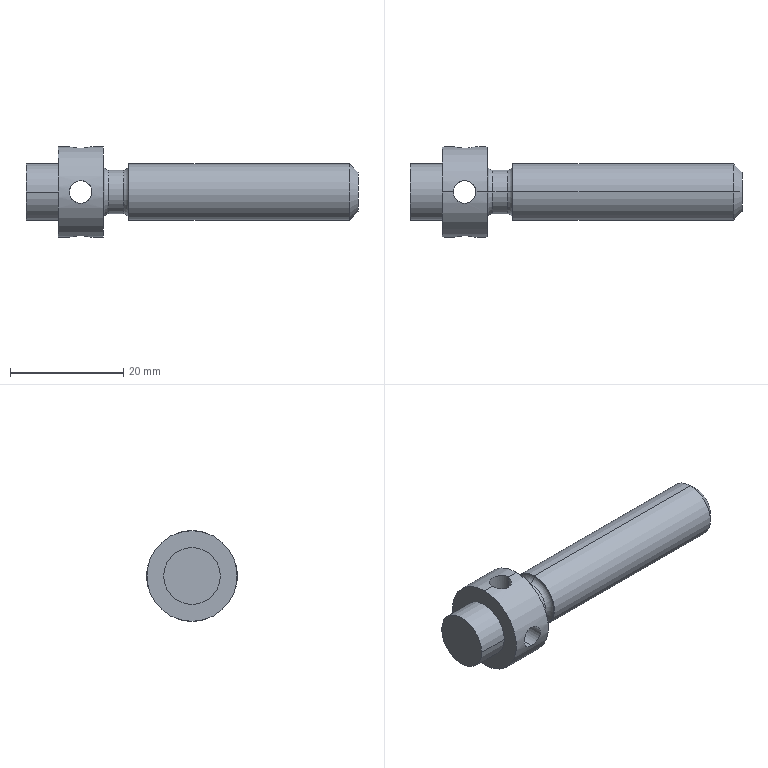Part | SolidWorks | features Boss 2, Cut 2, Chamfer 1, Extrusion 1, Fillet 1, ICE 1, Revolution 1 | 1 solid | 27 faces | box 58.66 x 16 x 16 mm | volume 5066 mm3 | cylinder 16 | plane 5 | torus 4 | cone 2 | commonest cylinder face diameters 4 x8 10 x4 7.7 x2 16 x2
STEP:
#1=CARTESIAN_POINT('',(-40.5,0.,4.85));
#2=VERTEX_POINT('',#1);
#3=CARTESIAN_POINT('',(-40.5,0.,-4.85));
#4=VERTEX_POINT('',#3);
#5=CARTESIAN_POINT('',(-40.5,0.,0.));
#6=DIRECTION('',(1.,0.,0.));
#7=DIRECTION('',(0.,0.,-1.));
#8=AXIS2_PLACEMENT_3D('',#5,#6,#7);
#9=CIRCLE('',#8,4.85);
#10=EDGE_CURVE('',#2,#4,#9,.T.);
#11=ORIENTED_EDGE('',*,*,#10,.F.);
#12=CARTESIAN_POINT('',(-41.5,0.,3.85));
#13=VERTEX_POINT('',#12);
#14=CARTESIAN_POINT('',(-41.5,0.,4.85));
#15=DIRECTION('',(0.,1.,0.));
#16=DIRECTION('',(0.,0.,1.));
#17=AXIS2_PLACEMENT_3D('',#14,#15,#16);
#18=CIRCLE('',#17,1.);
#19=EDGE_CURVE('',#2,#13,#18,.T.);
#20=ORIENTED_EDGE('',*,*,#19,.T.);
#21=CARTESIAN_POINT('',(-41.5,0.,-3.85));
#22=VERTEX_POINT('',#21);
#23=CARTESIAN_POINT('',(-41.5,0.,0.));
#24=DIRECTION('',(-1.,0.,0.));
#25=DIRECTION('',(0.,0.,-1.));
#26=AXIS2_PLACEMENT_3D('',#23,#24,#25);
#27=CIRCLE('',#26,3.85);
#28=EDGE_CURVE('',#22,#13,#27,.T.);
#29=ORIENTED_EDGE('',*,*,#28,.F.);
#30=CARTESIAN_POINT('',(-41.5,0.,-4.85));
#31=DIRECTION('',(0.,-1.,0.));
#32=DIRECTION('',(1.,0.,0.));
#33=AXIS2_PLACEMENT_3D('',#30,#31,#32);
#34=CIRCLE('',#33,1.);
#35=EDGE_CURVE('',#4,#22,#34,.T.);
#36=ORIENTED_EDGE('',*,*,#35,.F.);
#37=EDGE_LOOP('',(#11,#20,#29,#36));
#38=FACE_OUTER_BOUND('',#37,.T.);
#39=CARTESIAN_POINT('',(-41.5,0.,0.));
#40=DIRECTION('',(1.,0.,0.));
#41=DIRECTION('',(0.,0.,-1.));
#42=AXIS2_PLACEMENT_3D('',#39,#40,#41);
#43=TOROIDAL_SURFACE('',#42,4.85,1.);
#44=ADVANCED_FACE('',(#38),#43,.F.);
#45=CARTESIAN_POINT('',(-45.,0.,-4.85));
#46=VERTEX_POINT('',#45);
#47=CARTESIAN_POINT('',(-45.,0.,4.85));
#48=VERTEX_POINT('',#47);
#49=CARTESIAN_POINT('',(-45.,0.,0.));
#50=DIRECTION('',(-1.,0.,0.));
#51=DIRECTION('',(0.,0.,1.));
#52=AXIS2_PLACEMENT_3D('',#49,#50,#51);
#53=CIRCLE('',#52,4.85);
#54=EDGE_CURVE('',#46,#48,#53,.T.);
#55=ORIENTED_EDGE('',*,*,#54,.F.);
#56=CARTESIAN_POINT('',(-44.,0.,-3.85));
#57=VERTEX_POINT('',#56);
#58=CARTESIAN_POINT('',(-44.,0.,-4.85));
#59=DIRECTION('',(0.,1.,0.));
#60=DIRECTION('',(0.,0.,1.));
#61=AXIS2_PLACEMENT_3D('',#58,#59,#60);
#62=CIRCLE('',#61,1.);
#63=EDGE_CURVE('',#46,#57,#62,.T.);
#64=ORIENTED_EDGE('',*,*,#63,.T.);
#65=CARTESIAN_POINT('',(-44.,0.,3.85));
#66=VERTEX_POINT('',#65);
#67=CARTESIAN_POINT('',(-44.,0.,0.));
#68=DIRECTION('',(1.,0.,0.));
#69=DIRECTION('',(0.,0.,1.));
#70=AXIS2_PLACEMENT_3D('',#67,#68,#69);
#71=CIRCLE('',#70,3.85);
#72=EDGE_CURVE('',#66,#57,#71,.T.);
#73=ORIENTED_EDGE('',*,*,#72,.F.);
#74=CARTESIAN_POINT('',(-44.,0.,4.85));
#75=DIRECTION('',(0.,-1.,0.));
#76=DIRECTION('',(1.,0.,0.));
#77=AXIS2_PLACEMENT_3D('',#74,#75,#76);
#78=CIRCLE('',#77,1.);
#79=EDGE_CURVE('',#48,#66,#78,.T.);
#80=ORIENTED_EDGE('',*,*,#79,.F.);
#81=EDGE_LOOP('',(#55,#64,#73,#80));
#82=FACE_OUTER_BOUND('',#81,.T.);
#83=CARTESIAN_POINT('',(-44.,0.,0.));
#84=DIRECTION('',(-1.,0.,0.));
#85=DIRECTION('',(0.,0.,1.));
#86=AXIS2_PLACEMENT_3D('',#83,#84,#85);
#87=TOROIDAL_SURFACE('',#86,4.85,1.);
#88=ADVANCED_FACE('',(#82),#87,.F.);
#89=CARTESIAN_POINT('',(-58.66,-5.,0.));
#90=VERTEX_POINT('',#89);
#91=CARTESIAN_POINT('',(-58.66,5.,0.));
#92=VERTEX_POINT('',#91);
#93=CARTESIAN_POINT('',(-58.66,0.,0.));
#94=DIRECTION('',(-1.,0.,0.));
#95=DIRECTION('',(0.,0.,-1.));
#96=AXIS2_PLACEMENT_3D('',#93,#94,#95);
#97=CIRCLE('',#96,5.);
#98=EDGE_CURVE('',#90,#92,#97,.T.);
#99=ORIENTED_EDGE('',*,*,#98,.F.);
#100=CARTESIAN_POINT('',(-53.,-5.,0.));
#101=VERTEX_POINT('',#100);
#102=CARTESIAN_POINT('',(-53.,-5.,0.));
#103=DIRECTION('',(1.,0.,0.));
#104=VECTOR('',#103,1000.);
#105=LINE('',#102,#104);
#106=EDGE_CURVE('',#90,#101,#105,.T.);
#107=ORIENTED_EDGE('',*,*,#106,.T.);
#108=CARTESIAN_POINT('',(-53.,5.,0.));
#109=VERTEX_POINT('',#108);
#110=CARTESIAN_POINT('',(-53.,0.,0.));
#111=DIRECTION('',(-1.,0.,0.));
#112=DIRECTION('',(0.,0.,1.));
#113=AXIS2_PLACEMENT_3D('',#110,#111,#112);
#114=CIRCLE('',#113,5.);
#115=EDGE_CURVE('',#101,#109,#114,.T.);
#116=ORIENTED_EDGE('',*,*,#115,.T.);
#117=CARTESIAN_POINT('',(-53.,5.,0.));
#118=DIRECTION('',(1.,0.,0.));
#119=VECTOR('',#118,1000.);
#120=LINE('',#117,#119);
#121=EDGE_CURVE('',#92,#109,#120,.T.);
#122=ORIENTED_EDGE('',*,*,#121,.F.);
#123=EDGE_LOOP('',(#99,#107,#116,#122));
#124=FACE_OUTER_BOUND('',#123,.T.);
#125=CARTESIAN_POINT('',(-53.,0.,0.));
#126=DIRECTION('',(1.,0.,0.));
#127=DIRECTION('',(0.,1.,0.));
#128=AXIS2_PLACEMENT_3D('',#125,#126,#127);
#129=CYLINDRICAL_SURFACE('',#128,5.);
#130=ADVANCED_FACE('',(#124),#129,.T.);
#131=CARTESIAN_POINT('',(-49.,-7.746,-2.));
#132=VERTEX_POINT('',#131);
#133=CARTESIAN_POINT('',(-49.,-7.746,2.));
#134=VERTEX_POINT('',#133);
#135=CARTESIAN_POINT('',(-49.,-7.746,-2.));
#136=CARTESIAN_POINT('',(-49.131,-7.746,-2.));
#137=CARTESIAN_POINT('',(-49.264,-7.749,-1.987));
#138=CARTESIAN_POINT('',(-49.521,-7.762,-1.935));
#139=CARTESIAN_POINT('',(-49.646,-7.772,-1.897));
#140=CARTESIAN_POINT('',(-50.01,-7.808,-1.746));
#141=CARTESIAN_POINT('',(-50.23,-7.841,-1.599));
#142=CARTESIAN_POINT('',(-50.508,-7.891,-1.321));
#143=CARTESIAN_POINT('',(-50.59,-7.907,-1.22));
#144=CARTESIAN_POINT('',(-50.735,-7.937,-1.004));
#145=CARTESIAN_POINT('',(-50.797,-7.952,-0.887));
#146=CARTESIAN_POINT('',(-50.897,-7.975,-0.6456));
#147=CARTESIAN_POINT('',(-50.935,-7.984,-0.5209));
#148=CARTESIAN_POINT('',(-50.987,-7.997,-0.2633));
#149=CARTESIAN_POINT('',(-51.,-8.,-0.1305));
#150=CARTESIAN_POINT('',(-51.,-8.,0.2619));
#151=CARTESIAN_POINT('',(-50.947,-7.986,0.5261));
#152=CARTESIAN_POINT('',(-50.797,-7.952,0.8874));
#153=CARTESIAN_POINT('',(-50.734,-7.937,1.004));
#154=CARTESIAN_POINT('',(-50.589,-7.907,1.221));
#155=CARTESIAN_POINT('',(-50.507,-7.891,1.322));
#156=CARTESIAN_POINT('',(-50.322,-7.857,1.506));
#157=CARTESIAN_POINT('',(-50.22,-7.841,1.59));
#158=CARTESIAN_POINT('',(-50.004,-7.81,1.735));
#159=CARTESIAN_POINT('',(-49.889,-7.796,1.796));
#160=CARTESIAN_POINT('',(-49.524,-7.76,1.948));
#161=CARTESIAN_POINT('',(-49.264,-7.746,2.));
#162=CARTESIAN_POINT('',(-49.,-7.746,2.));
#163=B_SPLINE_CURVE_WITH_KNOTS('',3,(#135,#136,#137,#138,#139,#140,#141,#142,#143,#144,#145,#146,#147,#148,#149,#150,#151,#152,#153,#154,#155,#156,#157,#158,#159,#160,#161,#162),.UNSPECIFIED.,.F.,.F.,(4,2,2,2,2,2,2,2,2,2,2,2,2,4),(0.00314,0.003532,0.003924,0.004709,0.005101,0.005494,0.005886,0.006278,0.007063,0.007455,0.007847,0.00824,0.008632,0.009417),.UNSPECIFIED.);
#164=EDGE_CURVE('',#132,#134,#163,.T.);
#165=ORIENTED_EDGE('',*,*,#164,.F.);
#166=CARTESIAN_POINT('',(-49.,-2.,-2.));
#167=VERTEX_POINT('',#166);
#168=CARTESIAN_POINT('',(-49.,-8.,-2.));
#169=DIRECTION('',(0.,1.,0.));
#170=VECTOR('',#169,1000.);
#171=LINE('',#168,#170);
#172=EDGE_CURVE('',#132,#167,#171,.T.);
#173=ORIENTED_EDGE('',*,*,#172,.T.);
#174=CARTESIAN_POINT('',(-51.,0.,0.));
#175=VERTEX_POINT('',#174);
#176=CARTESIAN_POINT('',(-51.,0.,0.));
#177=CARTESIAN_POINT('',(-51.,-1.172,-1.172));
#178=CARTESIAN_POINT('',(-50.172,-2.,-2.));
#179=CARTESIAN_POINT('',(-49.,-2.,-2.));
#180=(BOUNDED_CURVE()B_SPLINE_CURVE(3,(#176,#177,#178,#179),.UNSPECIFIED.,.F.,.T.)B_SPLINE_CURVE_WITH_KNOTS((4,4),(1.571,3.142),.UNSPECIFIED.)CURVE()GEOMETRIC_REPRESENTATION_ITEM()RATIONAL_B_SPLINE_CURVE((1.,0.8047,0.8047,1.))REPRESENTATION_ITEM(''));
#181=EDGE_CURVE('',#175,#167,#180,.T.);
#182=ORIENTED_EDGE('',*,*,#181,.F.);
#183=CARTESIAN_POINT('',(-49.,-2.,2.));
#184=VERTEX_POINT('',#183);
#185=CARTESIAN_POINT('',(-49.,-2.,2.));
#186=CARTESIAN_POINT('',(-50.172,-2.,2.));
#187=CARTESIAN_POINT('',(-51.,-1.172,1.172));
#188=CARTESIAN_POINT('',(-51.,0.,0.));
#189=(BOUNDED_CURVE()B_SPLINE_CURVE(3,(#185,#186,#187,#188),.UNSPECIFIED.,.F.,.F.)B_SPLINE_CURVE_WITH_KNOTS((4,4),(0.,1.571),.UNSPECIFIED.)CURVE()GEOMETRIC_REPRESENTATION_ITEM()RATIONAL_B_SPLINE_CURVE((1.,0.8047,0.8047,1.))REPRESENTATION_ITEM(''));
#190=EDGE_CURVE('',#184,#175,#189,.T.);
#191=ORIENTED_EDGE('',*,*,#190,.F.);
#192=CARTESIAN_POINT('',(-49.,-8.,2.));
#193=DIRECTION('',(0.,1.,0.));
#194=VECTOR('',#193,1000.);
#195=LINE('',#192,#194);
#196=EDGE_CURVE('',#134,#184,#195,.T.);
#197=ORIENTED_EDGE('',*,*,#196,.F.);
#198=EDGE_LOOP('',(#165,#173,#182,#191,#197));
#199=FACE_OUTER_BOUND('',#198,.T.);
#200=CARTESIAN_POINT('',(-49.,-8.,0.));
#201=DIRECTION('',(0.,1.,0.));
#202=DIRECTION('',(0.,0.,1.));
#203=AXIS2_PLACEMENT_3D('',#200,#201,#202);
#204=CYLINDRICAL_SURFACE('',#203,2.);
#205=ADVANCED_FACE('',(#199),#204,.F.);
#206=CARTESIAN_POINT('',(-49.,2.,-2.));
#207=VERTEX_POINT('',#206);
#208=CARTESIAN_POINT('',(-49.,2.,-2.));
#209=CARTESIAN_POINT('',(-50.172,2.,-2.));
#210=CARTESIAN_POINT('',(-51.,1.172,-1.172));
#211=CARTESIAN_POINT('',(-51.,0.,0.));
#212=(BOUNDED_CURVE()B_SPLINE_CURVE(3,(#208,#209,#210,#211),.UNSPECIFIED.,.F.,.F.)B_SPLINE_CURVE_WITH_KNOTS((4,4),(3.142,4.712),.UNSPECIFIED.)CURVE()GEOMETRIC_REPRESENTATION_ITEM()RATIONAL_B_SPLINE_CURVE((1.,0.8047,0.8047,1.))REPRESENTATION_ITEM(''));
#213=EDGE_CURVE('',#207,#175,#212,.T.);
#214=ORIENTED_EDGE('',*,*,#213,.F.);
#215=CARTESIAN_POINT('',(-49.,7.746,-2.));
#216=VERTEX_POINT('',#215);
#217=CARTESIAN_POINT('',(-49.,-8.,-2.));
#218=DIRECTION('',(0.,1.,0.));
#219=VECTOR('',#218,1000.);
#220=LINE('',#217,#219);
#221=EDGE_CURVE('',#207,#216,#220,.T.);
#222=ORIENTED_EDGE('',*,*,#221,.T.);
#223=CARTESIAN_POINT('',(-49.,7.746,2.));
#224=VERTEX_POINT('',#223);
#225=CARTESIAN_POINT('',(-49.,7.746,2.));
#226=CARTESIAN_POINT('',(-49.133,7.746,2.));
#227=CARTESIAN_POINT('',(-49.263,7.749,1.987));
#228=CARTESIAN_POINT('',(-49.519,7.762,1.936));
#229=CARTESIAN_POINT('',(-49.647,7.772,1.897));
#230=CARTESIAN_POINT('',(-49.889,7.796,1.796));
#231=CARTESIAN_POINT('',(-50.003,7.81,1.735));
#232=CARTESIAN_POINT('',(-50.22,7.841,1.59));
#233=CARTESIAN_POINT('',(-50.323,7.858,1.506));
#234=CARTESIAN_POINT('',(-50.598,7.907,1.23));
#235=CARTESIAN_POINT('',(-50.747,7.94,1.008));
#236=CARTESIAN_POINT('',(-50.897,7.975,0.6471));
#237=CARTESIAN_POINT('',(-50.936,7.984,0.5204));
#238=CARTESIAN_POINT('',(-50.987,7.997,0.262));
#239=CARTESIAN_POINT('',(-51.,8.,0.1319));
#240=CARTESIAN_POINT('',(-51.,8.,-0.1302));
#241=CARTESIAN_POINT('',(-50.987,7.997,-0.2634));
#242=CARTESIAN_POINT('',(-50.936,7.984,-0.5203));
#243=CARTESIAN_POINT('',(-50.898,7.975,-0.6453));
#244=CARTESIAN_POINT('',(-50.746,7.94,-1.01));
#245=CARTESIAN_POINT('',(-50.599,7.907,-1.229));
#246=CARTESIAN_POINT('',(-50.321,7.857,-1.507));
#247=CARTESIAN_POINT('',(-50.221,7.841,-1.59));
#248=CARTESIAN_POINT('',(-50.004,7.81,-1.734));
#249=CARTESIAN_POINT('',(-49.887,7.796,-1.797));
#250=CARTESIAN_POINT('',(-49.646,7.772,-1.897));
#251=CARTESIAN_POINT('',(-49.521,7.762,-1.935));
#252=CARTESIAN_POINT('',(-49.264,7.749,-1.987));
#253=CARTESIAN_POINT('',(-49.131,7.746,-2.));
#254=CARTESIAN_POINT('',(-49.,7.746,-2.));
#255=B_SPLINE_CURVE_WITH_KNOTS('',3,(#225,#226,#227,#228,#229,#230,#231,#232,#233,#234,#235,#236,#237,#238,#239,#240,#241,#242,#243,#244,#245,#246,#247,#248,#249,#250,#251,#252,#253,#254),.UNSPECIFIED.,.F.,.F.,(4,2,2,2,2,2,2,2,2,2,2,2,2,2,4),(0.,0.0003924,0.0007847,0.001177,0.001569,0.002354,0.002747,0.003139,0.003531,0.003924,0.004708,0.005101,0.005493,0.005885,0.006278),.UNSPECIFIED.);
#256=EDGE_CURVE('',#224,#216,#255,.T.);
#257=ORIENTED_EDGE('',*,*,#256,.F.);
#258=CARTESIAN_POINT('',(-49.,2.,2.));
#259=VERTEX_POINT('',#258);
#260=CARTESIAN_POINT('',(-49.,-8.,2.));
#261=DIRECTION('',(0.,1.,0.));
#262=VECTOR('',#261,1000.);
#263=LINE('',#260,#262);
#264=EDGE_CURVE('',#259,#224,#263,.T.);
#265=ORIENTED_EDGE('',*,*,#264,.F.);
#266=CARTESIAN_POINT('',(-51.,0.,0.));
#267=CARTESIAN_POINT('',(-51.,1.172,1.172));
#268=CARTESIAN_POINT('',(-50.172,2.,2.));
#269=CARTESIAN_POINT('',(-49.,2.,2.));
#270=(BOUNDED_CURVE()B_SPLINE_CURVE(3,(#266,#267,#268,#269),.UNSPECIFIED.,.F.,.F.)B_SPLINE_CURVE_WITH_KNOTS((4,4),(4.712,6.283),.UNSPECIFIED.)CURVE()GEOMETRIC_REPRESENTATION_ITEM()RATIONAL_B_SPLINE_CURVE((1.,0.8047,0.8047,1.))REPRESENTATION_ITEM(''));
#271=EDGE_CURVE('',#175,#259,#270,.T.);
#272=ORIENTED_EDGE('',*,*,#271,.F.);
#273=EDGE_LOOP('',(#214,#222,#257,#265,#272));
#274=FACE_OUTER_BOUND('',#273,.T.);
#275=CARTESIAN_POINT('',(-49.,-8.,0.));
#276=DIRECTION('',(0.,1.,0.));
#277=DIRECTION('',(0.,0.,1.));
#278=AXIS2_PLACEMENT_3D('',#275,#276,#277);
#279=CYLINDRICAL_SURFACE('',#278,2.);
#280=ADVANCED_FACE('',(#274),#279,.F.);
#281=CARTESIAN_POINT('',(-51.,0.,-8.));
#282=VERTEX_POINT('',#281);
#283=CARTESIAN_POINT('',(-47.,0.,-8.));
#284=VERTEX_POINT('',#283);
#285=CARTESIAN_POINT('',(-51.,0.,-8.));
#286=CARTESIAN_POINT('',(-51.,-0.2616,-8.));
#287=CARTESIAN_POINT('',(-50.947,-0.5257,-7.986));
#288=CARTESIAN_POINT('',(-50.797,-0.8871,-7.952));
#289=CARTESIAN_POINT('',(-50.735,-1.004,-7.937));
#290=CARTESIAN_POINT('',(-50.589,-1.221,-7.907));
#291=CARTESIAN_POINT('',(-50.507,-1.321,-7.891));
#292=CARTESIAN_POINT('',(-50.323,-1.506,-7.858));
#293=CARTESIAN_POINT('',(-50.22,-1.59,-7.841));
#294=CARTESIAN_POINT('',(-50.004,-1.734,-7.81));
#295=CARTESIAN_POINT('',(-49.89,-1.796,-7.796));
#296=CARTESIAN_POINT('',(-49.525,-1.948,-7.76));
#297=CARTESIAN_POINT('',(-49.264,-2.,-7.746));
#298=CARTESIAN_POINT('',(-48.869,-2.,-7.746));
#299=CARTESIAN_POINT('',(-48.739,-1.987,-7.749));
#300=CARTESIAN_POINT('',(-48.482,-1.936,-7.762));
#301=CARTESIAN_POINT('',(-48.354,-1.897,-7.772));
#302=CARTESIAN_POINT('',(-47.992,-1.747,-7.808));
#303=CARTESIAN_POINT('',(-47.77,-1.598,-7.841));
#304=CARTESIAN_POINT('',(-47.403,-1.232,-7.907));
#305=CARTESIAN_POINT('',(-47.254,-1.01,-7.94));
#306=CARTESIAN_POINT('',(-47.104,-0.6486,-7.975));
#307=CARTESIAN_POINT('',(-47.065,-0.5212,-7.984));
#308=CARTESIAN_POINT('',(-47.013,-0.2634,-7.997));
#309=CARTESIAN_POINT('',(-47.,-0.1327,-8.));
#310=CARTESIAN_POINT('',(-47.,0.,-8.));
#311=B_SPLINE_CURVE_WITH_KNOTS('',3,(#285,#286,#287,#288,#289,#290,#291,#292,#293,#294,#295,#296,#297,#298,#299,#300,#301,#302,#303,#304,#305,#306,#307,#308,#309,#310),.UNSPECIFIED.,.F.,.F.,(4,2,2,2,2,2,2,2,2,2,2,2,4),(0.006278,0.007062,0.007455,0.007847,0.008239,0.008631,0.009416,0.009808,0.0102,0.01099,0.01177,0.01216,0.01255),.UNSPECIFIED.);
#312=EDGE_CURVE('',#282,#284,#311,.T.);
#313=ORIENTED_EDGE('',*,*,#312,.F.);
#314=CARTESIAN_POINT('',(-51.,0.,-8.));
#315=DIRECTION('',(0.,0.,1.));
#316=VECTOR('',#315,1000.);
#317=LINE('',#314,#316);
#318=EDGE_CURVE('',#282,#175,#317,.T.);
#319=ORIENTED_EDGE('',*,*,#318,.T.);
#320=ORIENTED_EDGE('',*,*,#181,.T.);
#321=CARTESIAN_POINT('',(-47.,0.,0.));
#322=VERTEX_POINT('',#321);
#323=CARTESIAN_POINT('',(-49.,-2.,-2.));
#324=CARTESIAN_POINT('',(-47.828,-2.,-2.));
#325=CARTESIAN_POINT('',(-47.,-1.172,-1.172));
#326=CARTESIAN_POINT('',(-47.,0.,0.));
#327=(BOUNDED_CURVE()B_SPLINE_CURVE(3,(#323,#324,#325,#326),.UNSPECIFIED.,.F.,.T.)B_SPLINE_CURVE_WITH_KNOTS((4,4),(3.142,4.712),.UNSPECIFIED.)CURVE()GEOMETRIC_REPRESENTATION_ITEM()RATIONAL_B_SPLINE_CURVE((1.,0.8047,0.8047,1.))REPRESENTATION_ITEM(''));
#328=EDGE_CURVE('',#167,#322,#327,.T.);
#329=ORIENTED_EDGE('',*,*,#328,.T.);
#330=CARTESIAN_POINT('',(-47.,0.,-8.));
#331=DIRECTION('',(0.,0.,1.));
#332=VECTOR('',#331,1000.);
#333=LINE('',#330,#332);
#334=EDGE_CURVE('',#284,#322,#333,.T.);
#335=ORIENTED_EDGE('',*,*,#334,.F.);
#336=EDGE_LOOP('',(#313,#319,#320,#329,#335));
#337=FACE_OUTER_BOUND('',#336,.T.);
#338=CARTESIAN_POINT('',(-49.,0.,-8.));
#339=DIRECTION('',(0.,0.,1.));
#340=DIRECTION('',(1.,0.,0.));
#341=AXIS2_PLACEMENT_3D('',#338,#339,#340);
#342=CYLINDRICAL_SURFACE('',#341,2.);
#343=ADVANCED_FACE('',(#337),#342,.F.);
#344=ORIENTED_EDGE('',*,*,#256,.T.);
#345=CARTESIAN_POINT('',(-49.,7.746,-2.));
#346=CARTESIAN_POINT('',(-48.738,7.746,-2.));
#347=CARTESIAN_POINT('',(-48.474,7.76,-1.947));
#348=CARTESIAN_POINT('',(-48.113,7.796,-1.797));
#349=CARTESIAN_POINT('',(-47.996,7.81,-1.735));
#350=CARTESIAN_POINT('',(-47.779,7.841,-1.589));
#351=CARTESIAN_POINT('',(-47.679,7.857,-1.507));
#352=CARTESIAN_POINT('',(-47.494,7.89,-1.323));
#353=CARTESIAN_POINT('',(-47.41,7.907,-1.22));
#354=CARTESIAN_POINT('',(-47.266,7.937,-1.004));
#355=CARTESIAN_POINT('',(-47.204,7.951,-0.8897));
#356=CARTESIAN_POINT('',(-47.052,7.987,-0.5248));
#357=CARTESIAN_POINT('',(-47.,8.,-0.2644));
#358=CARTESIAN_POINT('',(-47.,8.,0.1313));
#359=CARTESIAN_POINT('',(-47.013,7.997,0.2615));
#360=CARTESIAN_POINT('',(-47.064,7.984,0.5184));
#361=CARTESIAN_POINT('',(-47.103,7.975,0.646));
#362=CARTESIAN_POINT('',(-47.253,7.94,1.008));
#363=CARTESIAN_POINT('',(-47.402,7.907,1.23));
#364=CARTESIAN_POINT('',(-47.769,7.841,1.597));
#365=CARTESIAN_POINT('',(-47.99,7.808,1.746));
#366=CARTESIAN_POINT('',(-48.351,7.772,1.896));
#367=CARTESIAN_POINT('',(-48.479,7.762,1.935));
#368=CARTESIAN_POINT('',(-48.737,7.749,1.987));
#369=CARTESIAN_POINT('',(-48.867,7.746,2.));
#370=CARTESIAN_POINT('',(-49.,7.746,2.));
#371=B_SPLINE_CURVE_WITH_KNOTS('',3,(#345,#346,#347,#348,#349,#350,#351,#352,#353,#354,#355,#356,#357,#358,#359,#360,#361,#362,#363,#364,#365,#366,#367,#368,#369,#370),.UNSPECIFIED.,.F.,.F.,(4,2,2,2,2,2,2,2,2,2,2,2,4),(0.006278,0.007062,0.007455,0.007847,0.008239,0.008631,0.009416,0.009808,0.0102,0.01098,0.01177,0.01216,0.01255),.UNSPECIFIED.);
#372=EDGE_CURVE('',#216,#224,#371,.T.);
#373=ORIENTED_EDGE('',*,*,#372,.T.);
#374=EDGE_LOOP('',(#344,#373));
#375=FACE_BOUND('',#374,.T.);
#376=CARTESIAN_POINT('',(-53.,0.,8.));
#377=VERTEX_POINT('',#376);
#378=CARTESIAN_POINT('',(-53.,0.,-8.));
#379=VERTEX_POINT('',#378);
#380=CARTESIAN_POINT('',(-53.,0.,0.));
#381=DIRECTION('',(-1.,0.,0.));
#382=DIRECTION('',(0.,0.,1.));
#383=AXIS2_PLACEMENT_3D('',#380,#381,#382);
#384=CIRCLE('',#383,8.);
#385=EDGE_CURVE('',#377,#379,#384,.T.);
#386=ORIENTED_EDGE('',*,*,#385,.F.);
#387=CARTESIAN_POINT('',(-51.,0.,8.));
#388=VERTEX_POINT('',#387);
#389=CARTESIAN_POINT('',(-53.,0.,8.));
#390=DIRECTION('',(1.,0.,0.));
#391=VECTOR('',#390,1000.);
#392=LINE('',#389,#391);
#393=EDGE_CURVE('',#377,#388,#392,.T.);
#394=ORIENTED_EDGE('',*,*,#393,.T.);
#395=CARTESIAN_POINT('',(-47.,0.,8.));
#396=VERTEX_POINT('',#395);
#397=CARTESIAN_POINT('',(-51.,0.,8.));
#398=CARTESIAN_POINT('',(-51.,0.2616,8.));
#399=CARTESIAN_POINT('',(-50.947,0.5257,7.986));
#400=CARTESIAN_POINT('',(-50.797,0.8871,7.952));
#401=CARTESIAN_POINT('',(-50.735,1.004,7.937));
#402=CARTESIAN_POINT('',(-50.589,1.221,7.907));
#403=CARTESIAN_POINT('',(-50.507,1.321,7.891));
#404=CARTESIAN_POINT('',(-50.323,1.506,7.858));
#405=CARTESIAN_POINT('',(-50.22,1.59,7.841));
#406=CARTESIAN_POINT('',(-50.004,1.734,7.81));
#407=CARTESIAN_POINT('',(-49.89,1.796,7.796));
#408=CARTESIAN_POINT('',(-49.525,1.948,7.76));
#409=CARTESIAN_POINT('',(-49.264,2.,7.746));
#410=CARTESIAN_POINT('',(-48.869,2.,7.746));
#411=CARTESIAN_POINT('',(-48.739,1.987,7.749));
#412=CARTESIAN_POINT('',(-48.482,1.936,7.762));
#413=CARTESIAN_POINT('',(-48.354,1.897,7.772));
#414=CARTESIAN_POINT('',(-47.992,1.747,7.808));
#415=CARTESIAN_POINT('',(-47.77,1.598,7.841));
#416=CARTESIAN_POINT('',(-47.403,1.232,7.907));
#417=CARTESIAN_POINT('',(-47.254,1.01,7.94));
#418=CARTESIAN_POINT('',(-47.104,0.6486,7.975));
#419=CARTESIAN_POINT('',(-47.065,0.5212,7.984));
#420=CARTESIAN_POINT('',(-47.013,0.2634,7.997));
#421=CARTESIAN_POINT('',(-47.,0.1327,8.));
#422=CARTESIAN_POINT('',(-47.,0.,8.));
#423=B_SPLINE_CURVE_WITH_KNOTS('',3,(#397,#398,#399,#400,#401,#402,#403,#404,#405,#406,#407,#408,#409,#410,#411,#412,#413,#414,#415,#416,#417,#418,#419,#420,#421,#422),.UNSPECIFIED.,.F.,.F.,(4,2,2,2,2,2,2,2,2,2,2,2,4),(0.006278,0.007062,0.007455,0.007847,0.008239,0.008631,0.009416,0.009808,0.0102,0.01099,0.01177,0.01216,0.01255),.UNSPECIFIED.);
#424=EDGE_CURVE('',#388,#396,#423,.T.);
#425=ORIENTED_EDGE('',*,*,#424,.T.);
#426=CARTESIAN_POINT('',(-45.,0.,8.));
#427=VERTEX_POINT('',#426);
#428=CARTESIAN_POINT('',(-53.,0.,8.));
#429=DIRECTION('',(1.,0.,0.));
#430=VECTOR('',#429,1000.);
#431=LINE('',#428,#430);
#432=EDGE_CURVE('',#396,#427,#431,.T.);
#433=ORIENTED_EDGE('',*,*,#432,.T.);
#434=CARTESIAN_POINT('',(-45.,0.,-8.));
#435=VERTEX_POINT('',#434);
#436=CARTESIAN_POINT('',(-45.,0.,0.));
#437=DIRECTION('',(-1.,0.,0.));
#438=DIRECTION('',(0.,0.,1.));
#439=AXIS2_PLACEMENT_3D('',#436,#437,#438);
#440=CIRCLE('',#439,8.);
#441=EDGE_CURVE('',#427,#435,#440,.T.);
#442=ORIENTED_EDGE('',*,*,#441,.T.);
#443=CARTESIAN_POINT('',(-53.,0.,-8.));
#444=DIRECTION('',(1.,0.,0.));
#445=VECTOR('',#444,1000.);
#446=LINE('',#443,#445);
#447=EDGE_CURVE('',#284,#435,#446,.T.);
#448=ORIENTED_EDGE('',*,*,#447,.F.);
#449=CARTESIAN_POINT('',(-47.,0.,-8.));
#450=CARTESIAN_POINT('',(-47.,0.1327,-8.));
#451=CARTESIAN_POINT('',(-47.013,0.2631,-7.997));
#452=CARTESIAN_POINT('',(-47.064,0.5195,-7.984));
#453=CARTESIAN_POINT('',(-47.103,0.6468,-7.975));
#454=CARTESIAN_POINT('',(-47.204,0.8888,-7.951));
#455=CARTESIAN_POINT('',(-47.265,1.003,-7.938));
#456=CARTESIAN_POINT('',(-47.41,1.22,-7.907));
#457=CARTESIAN_POINT('',(-47.494,1.323,-7.89));
#458=CARTESIAN_POINT('',(-47.77,1.598,-7.841));
#459=CARTESIAN_POINT('',(-47.992,1.747,-7.808));
#460=CARTESIAN_POINT('',(-48.353,1.897,-7.772));
#461=CARTESIAN_POINT('',(-48.48,1.936,-7.762));
#462=CARTESIAN_POINT('',(-48.738,1.987,-7.749));
#463=CARTESIAN_POINT('',(-48.868,2.,-7.746));
#464=CARTESIAN_POINT('',(-49.13,2.,-7.746));
#465=CARTESIAN_POINT('',(-49.263,1.987,-7.749));
#466=CARTESIAN_POINT('',(-49.52,1.936,-7.762));
#467=CARTESIAN_POINT('',(-49.645,1.898,-7.772));
#468=CARTESIAN_POINT('',(-50.009,1.746,-7.808));
#469=CARTESIAN_POINT('',(-50.229,1.599,-7.841));
#470=CARTESIAN_POINT('',(-50.507,1.321,-7.891));
#471=CARTESIAN_POINT('',(-50.59,1.221,-7.907));
#472=CARTESIAN_POINT('',(-50.734,1.005,-7.937));
#473=CARTESIAN_POINT('',(-50.797,0.8874,-7.952));
#474=CARTESIAN_POINT('',(-50.897,0.646,-7.975));
#475=CARTESIAN_POINT('',(-50.935,0.5212,-7.984));
#476=CARTESIAN_POINT('',(-50.987,0.2636,-7.997));
#477=CARTESIAN_POINT('',(-51.,0.1308,-8.));
#478=CARTESIAN_POINT('',(-51.,0.,-8.));
#479=B_SPLINE_CURVE_WITH_KNOTS('',3,(#449,#450,#451,#452,#453,#454,#455,#456,#457,#458,#459,#460,#461,#462,#463,#464,#465,#466,#467,#468,#469,#470,#471,#472,#473,#474,#475,#476,#477,#478),.UNSPECIFIED.,.F.,.F.,(4,2,2,2,2,2,2,2,2,2,2,2,2,2,4),(0.,0.0003924,0.0007847,0.001177,0.001569,0.002354,0.002747,0.003139,0.003531,0.003924,0.004708,0.005101,0.005493,0.005886,0.006278),.UNSPECIFIED.);
#480=EDGE_CURVE('',#284,#282,#479,.T.);
#481=ORIENTED_EDGE('',*,*,#480,.T.);
#482=CARTESIAN_POINT('',(-53.,0.,-8.));
#483=DIRECTION('',(1.,0.,0.));
#484=VECTOR('',#483,1000.);
#485=LINE('',#482,#484);
#486=EDGE_CURVE('',#379,#282,#485,.T.);
#487=ORIENTED_EDGE('',*,*,#486,.F.);
#488=EDGE_LOOP('',(#386,#394,#425,#433,#442,#448,#481,#487));
#489=FACE_OUTER_BOUND('',#488,.T.);
#490=CARTESIAN_POINT('',(-53.,0.,0.));
#491=DIRECTION('',(1.,0.,0.));
#492=DIRECTION('',(0.,0.,-1.));
#493=AXIS2_PLACEMENT_3D('',#490,#491,#492);
#494=CYLINDRICAL_SURFACE('',#493,8.);
#495=ADVANCED_FACE('',(#375,#489),#494,.T.);
#496=CARTESIAN_POINT('',(-44.,0.,0.));
#497=DIRECTION('',(1.,0.,0.));
#498=DIRECTION('',(0.,0.,1.));
#499=AXIS2_PLACEMENT_3D('',#496,#497,#498);
#500=CIRCLE('',#499,3.85);
#501=EDGE_CURVE('',#57,#66,#500,.T.);
#502=ORIENTED_EDGE('',*,*,#501,.T.);
#503=CARTESIAN_POINT('',(-45.,0.,3.85));
#504=DIRECTION('',(1.,0.,0.));
#505=VECTOR('',#504,1000.);
#506=LINE('',#503,#505);
#507=EDGE_CURVE('',#66,#13,#506,.T.);
#508=ORIENTED_EDGE('',*,*,#507,.T.);
#509=CARTESIAN_POINT('',(-41.5,0.,0.));
#510=DIRECTION('',(-1.,0.,0.));
#511=DIRECTION('',(0.,0.,-1.));
#512=AXIS2_PLACEMENT_3D('',#509,#510,#511);
#513=CIRCLE('',#512,3.85);
#514=EDGE_CURVE('',#13,#22,#513,.T.);
#515=ORIENTED_EDGE('',*,*,#514,.T.);
#516=CARTESIAN_POINT('',(-45.,0.,-3.85));
#517=DIRECTION('',(1.,0.,0.));
#518=VECTOR('',#517,1000.);
#519=LINE('',#516,#518);
#520=EDGE_CURVE('',#57,#22,#519,.T.);
#521=ORIENTED_EDGE('',*,*,#520,.F.);
#522=EDGE_LOOP('',(#502,#508,#515,#521));
#523=FACE_OUTER_BOUND('',#522,.T.);
#524=CARTESIAN_POINT('',(-45.,0.,0.));
#525=DIRECTION('',(1.,0.,0.));
#526=DIRECTION('',(0.,0.,-1.));
#527=AXIS2_PLACEMENT_3D('',#524,#525,#526);
#528=CYLINDRICAL_SURFACE('',#527,3.85);
#529=ADVANCED_FACE('',(#523),#528,.T.);
#530=CARTESIAN_POINT('',(0.,0.,-3.5));
#531=VERTEX_POINT('',#530);
#532=CARTESIAN_POINT('',(0.,0.,3.5));
#533=VERTEX_POINT('',#532);
#534=CARTESIAN_POINT('',(0.,0.,0.));
#535=DIRECTION('',(1.,0.,0.));
#536=DIRECTION('',(0.,0.,-1.));
#537=AXIS2_PLACEMENT_3D('',#534,#535,#536);
#538=CIRCLE('',#537,3.5);
#539=EDGE_CURVE('',#531,#533,#538,.T.);
#540=ORIENTED_EDGE('',*,*,#539,.F.);
#541=CARTESIAN_POINT('',(-1.5,0.,-5.));
#542=VERTEX_POINT('',#541);
#543=CARTESIAN_POINT('',(0.,0.,-3.5));
#544=DIRECTION('',(-0.7071,0.,-0.7071));
#545=VECTOR('',#544,1000.);
#546=LINE('',#543,#545);
#547=EDGE_CURVE('',#531,#542,#546,.T.);
#548=ORIENTED_EDGE('',*,*,#547,.T.);
#549=CARTESIAN_POINT('',(-1.5,0.,5.));
#550=VERTEX_POINT('',#549);
#551=CARTESIAN_POINT('',(-1.5,0.,0.));
#552=DIRECTION('',(-1.,0.,0.));
#553=DIRECTION('',(0.,0.,-1.));
#554=AXIS2_PLACEMENT_3D('',#551,#552,#553);
#555=CIRCLE('',#554,5.);
#556=EDGE_CURVE('',#550,#542,#555,.T.);
#557=ORIENTED_EDGE('',*,*,#556,.F.);
#558=CARTESIAN_POINT('',(0.,0.,3.5));
#559=DIRECTION('',(-0.7071,0.,0.7071));
#560=VECTOR('',#559,1000.);
#561=LINE('',#558,#560);
#562=EDGE_CURVE('',#533,#550,#561,.T.);
#563=ORIENTED_EDGE('',*,*,#562,.F.);
#564=EDGE_LOOP('',(#540,#548,#557,#563));
#565=FACE_OUTER_BOUND('',#564,.T.);
#566=CARTESIAN_POINT('',(0.,0.,0.));
#567=DIRECTION('',(-1.,0.,0.));
#568=DIRECTION('',(0.,0.,1.));
#569=AXIS2_PLACEMENT_3D('',#566,#567,#568);
#570=CONICAL_SURFACE('',#569,3.5,0.7854);
#571=ADVANCED_FACE('',(#565),#570,.T.);
#572=CARTESIAN_POINT('',(-40.5,0.,-5.));
#573=VERTEX_POINT('',#572);
#574=CARTESIAN_POINT('',(-40.5,0.,5.));
#575=VERTEX_POINT('',#574);
#576=CARTESIAN_POINT('',(-40.5,0.,0.));
#577=DIRECTION('',(1.,0.,0.));
#578=DIRECTION('',(0.,0.,-1.));
#579=AXIS2_PLACEMENT_3D('',#576,#577,#578);
#580=CIRCLE('',#579,5.);
#581=EDGE_CURVE('',#573,#575,#580,.T.);
#582=ORIENTED_EDGE('',*,*,#581,.T.);
#583=CARTESIAN_POINT('',(-40.5,0.,5.));
#584=DIRECTION('',(1.,0.,0.));
#585=VECTOR('',#584,1000.);
#586=LINE('',#583,#585);
#587=EDGE_CURVE('',#575,#550,#586,.T.);
#588=ORIENTED_EDGE('',*,*,#587,.T.);
#589=ORIENTED_EDGE('',*,*,#556,.T.);
#590=CARTESIAN_POINT('',(-40.5,0.,-5.));
#591=DIRECTION('',(1.,0.,0.));
#592=VECTOR('',#591,1000.);
#593=LINE('',#590,#592);
#594=EDGE_CURVE('',#573,#542,#593,.T.);
#595=ORIENTED_EDGE('',*,*,#594,.F.);
#596=EDGE_LOOP('',(#582,#588,#589,#595));
#597=FACE_OUTER_BOUND('',#596,.T.);
#598=CARTESIAN_POINT('',(-40.5,0.,0.));
#599=DIRECTION('',(1.,0.,0.));
#600=DIRECTION('',(0.,0.,-1.));
#601=AXIS2_PLACEMENT_3D('',#598,#599,#600);
#602=CYLINDRICAL_SURFACE('',#601,5.);
#603=ADVANCED_FACE('',(#597),#602,.T.);
#604=CARTESIAN_POINT('',(-47.,0.,0.));
#605=CARTESIAN_POINT('',(-47.,-1.172,1.172));
#606=CARTESIAN_POINT('',(-47.828,-2.,2.));
#607=CARTESIAN_POINT('',(-49.,-2.,2.));
#608=(BOUNDED_CURVE()B_SPLINE_CURVE(3,(#604,#605,#606,#607),.UNSPECIFIED.,.F.,.F.)B_SPLINE_CURVE_WITH_KNOTS((4,4),(4.712,6.283),.UNSPECIFIED.)CURVE()GEOMETRIC_REPRESENTATION_ITEM()RATIONAL_B_SPLINE_CURVE((1.,0.8047,0.8047,1.))REPRESENTATION_ITEM(''));
#609=EDGE_CURVE('',#322,#184,#608,.T.);
#610=ORIENTED_EDGE('',*,*,#609,.T.);
#611=ORIENTED_EDGE('',*,*,#190,.T.);
#612=CARTESIAN_POINT('',(-51.,0.,-8.));
#613=DIRECTION('',(0.,0.,1.));
#614=VECTOR('',#613,1000.);
#615=LINE('',#612,#614);
#616=EDGE_CURVE('',#175,#388,#615,.T.);
#617=ORIENTED_EDGE('',*,*,#616,.T.);
#618=CARTESIAN_POINT('',(-47.,0.,8.));
#619=CARTESIAN_POINT('',(-47.,-0.1327,8.));
#620=CARTESIAN_POINT('',(-47.013,-0.2631,7.997));
#621=CARTESIAN_POINT('',(-47.064,-0.5195,7.984));
#622=CARTESIAN_POINT('',(-47.103,-0.6468,7.975));
#623=CARTESIAN_POINT('',(-47.204,-0.8888,7.951));
#624=CARTESIAN_POINT('',(-47.265,-1.003,7.938));
#625=CARTESIAN_POINT('',(-47.41,-1.22,7.907));
#626=CARTESIAN_POINT('',(-47.494,-1.323,7.89));
#627=CARTESIAN_POINT('',(-47.77,-1.598,7.841));
#628=CARTESIAN_POINT('',(-47.992,-1.747,7.808));
#629=CARTESIAN_POINT('',(-48.353,-1.897,7.772));
#630=CARTESIAN_POINT('',(-48.48,-1.936,7.762));
#631=CARTESIAN_POINT('',(-48.738,-1.987,7.749));
#632=CARTESIAN_POINT('',(-48.868,-2.,7.746));
#633=CARTESIAN_POINT('',(-49.13,-2.,7.746));
#634=CARTESIAN_POINT('',(-49.263,-1.987,7.749));
#635=CARTESIAN_POINT('',(-49.52,-1.936,7.762));
#636=CARTESIAN_POINT('',(-49.645,-1.898,7.772));
#637=CARTESIAN_POINT('',(-50.009,-1.746,7.808));
#638=CARTESIAN_POINT('',(-50.229,-1.599,7.841));
#639=CARTESIAN_POINT('',(-50.507,-1.321,7.891));
#640=CARTESIAN_POINT('',(-50.59,-1.221,7.907));
#641=CARTESIAN_POINT('',(-50.734,-1.005,7.937));
#642=CARTESIAN_POINT('',(-50.797,-0.8874,7.952));
#643=CARTESIAN_POINT('',(-50.897,-0.646,7.975));
#644=CARTESIAN_POINT('',(-50.935,-0.5212,7.984));
#645=CARTESIAN_POINT('',(-50.987,-0.2636,7.997));
#646=CARTESIAN_POINT('',(-51.,-0.1308,8.));
#647=CARTESIAN_POINT('',(-51.,0.,8.));
#648=B_SPLINE_CURVE_WITH_KNOTS('',3,(#618,#619,#620,#621,#622,#623,#624,#625,#626,#627,#628,#629,#630,#631,#632,#633,#634,#635,#636,#637,#638,#639,#640,#641,#642,#643,#644,#645,#646,#647),.UNSPECIFIED.,.F.,.F.,(4,2,2,2,2,2,2,2,2,2,2,2,2,2,4),(0.,0.0003924,0.0007847,0.001177,0.001569,0.002354,0.002747,0.003139,0.003531,0.003924,0.004708,0.005101,0.005493,0.005886,0.006278),.UNSPECIFIED.);
#649=EDGE_CURVE('',#396,#388,#648,.T.);
#650=ORIENTED_EDGE('',*,*,#649,.F.);
#651=CARTESIAN_POINT('',(-47.,0.,-8.));
#652=DIRECTION('',(0.,0.,1.));
#653=VECTOR('',#652,1000.);
#654=LINE('',#651,#653);
#655=EDGE_CURVE('',#322,#396,#654,.T.);
#656=ORIENTED_EDGE('',*,*,#655,.F.);
#657=EDGE_LOOP('',(#610,#611,#617,#650,#656));
#658=FACE_OUTER_BOUND('',#657,.T.);
#659=CARTESIAN_POINT('',(-49.,0.,-8.));
#660=DIRECTION('',(0.,0.,1.));
#661=DIRECTION('',(1.,0.,0.));
#662=AXIS2_PLACEMENT_3D('',#659,#660,#661);
#663=CYLINDRICAL_SURFACE('',#662,2.);
#664=ADVANCED_FACE('',(#658),#663,.F.);
#665=ORIENTED_EDGE('',*,*,#616,.F.);
#666=ORIENTED_EDGE('',*,*,#271,.T.);
#667=CARTESIAN_POINT('',(-49.,2.,2.));
#668=CARTESIAN_POINT('',(-47.828,2.,2.));
#669=CARTESIAN_POINT('',(-47.,1.172,1.172));
#670=CARTESIAN_POINT('',(-47.,0.,0.));
#671=(BOUNDED_CURVE()B_SPLINE_CURVE(3,(#667,#668,#669,#670),.UNSPECIFIED.,.F.,.F.)B_SPLINE_CURVE_WITH_KNOTS((4,4),(0.,1.571),.UNSPECIFIED.)CURVE()GEOMETRIC_REPRESENTATION_ITEM()RATIONAL_B_SPLINE_CURVE((1.,0.8047,0.8047,1.))REPRESENTATION_ITEM(''));
#672=EDGE_CURVE('',#259,#322,#671,.T.);
#673=ORIENTED_EDGE('',*,*,#672,.T.);
#674=ORIENTED_EDGE('',*,*,#655,.T.);
#675=ORIENTED_EDGE('',*,*,#424,.F.);
#676=EDGE_LOOP('',(#665,#666,#673,#674,#675));
#677=FACE_OUTER_BOUND('',#676,.T.);
#678=CARTESIAN_POINT('',(-49.,0.,-8.));
#679=DIRECTION('',(0.,0.,1.));
#680=DIRECTION('',(1.,0.,0.));
#681=AXIS2_PLACEMENT_3D('',#678,#679,#680);
#682=CYLINDRICAL_SURFACE('',#681,2.);
#683=ADVANCED_FACE('',(#677),#682,.F.);
#684=CARTESIAN_POINT('',(-40.5,0.,0.));
#685=DIRECTION('',(1.,0.,0.));
#686=DIRECTION('',(0.,0.,-1.));
#687=AXIS2_PLACEMENT_3D('',#684,#685,#686);
#688=CIRCLE('',#687,4.85);
#689=EDGE_CURVE('',#4,#2,#688,.T.);
#690=ORIENTED_EDGE('',*,*,#689,.T.);
#691=ORIENTED_EDGE('',*,*,#10,.T.);
#692=EDGE_LOOP('',(#690,#691));
#693=FACE_BOUND('',#692,.T.);
#694=ORIENTED_EDGE('',*,*,#581,.F.);
#695=CARTESIAN_POINT('',(-40.5,0.,0.));
#696=DIRECTION('',(1.,0.,0.));
#697=DIRECTION('',(0.,0.,-1.));
#698=AXIS2_PLACEMENT_3D('',#695,#696,#697);
#699=CIRCLE('',#698,5.);
#700=EDGE_CURVE('',#575,#573,#699,.T.);
#701=ORIENTED_EDGE('',*,*,#700,.F.);
#702=EDGE_LOOP('',(#694,#701));
#703=FACE_OUTER_BOUND('',#702,.T.);
#704=CARTESIAN_POINT('',(-40.5,0.,0.));
#705=DIRECTION('',(1.,0.,0.));
#706=DIRECTION('',(0.,0.,-1.));
#707=AXIS2_PLACEMENT_3D('',#704,#705,#706);
#708=PLANE('',#707);
#709=ADVANCED_FACE('',(#693,#703),#708,.F.);
#710=ORIENTED_EDGE('',*,*,#587,.F.);
#711=ORIENTED_EDGE('',*,*,#700,.T.);
#712=ORIENTED_EDGE('',*,*,#594,.T.);
#713=CARTESIAN_POINT('',(-1.5,0.,0.));
#714=DIRECTION('',(-1.,0.,0.));
#715=DIRECTION('',(0.,0.,-1.));
#716=AXIS2_PLACEMENT_3D('',#713,#714,#715);
#717=CIRCLE('',#716,5.);
#718=EDGE_CURVE('',#542,#550,#717,.T.);
#719=ORIENTED_EDGE('',*,*,#718,.T.);
#720=EDGE_LOOP('',(#710,#711,#712,#719));
#721=FACE_OUTER_BOUND('',#720,.T.);
#722=CARTESIAN_POINT('',(-40.5,0.,0.));
#723=DIRECTION('',(1.,0.,0.));
#724=DIRECTION('',(0.,0.,-1.));
#725=AXIS2_PLACEMENT_3D('',#722,#723,#724);
#726=CYLINDRICAL_SURFACE('',#725,5.);
#727=ADVANCED_FACE('',(#721),#726,.T.);
#728=CARTESIAN_POINT('',(0.,0.,0.));
#729=DIRECTION('',(1.,0.,0.));
#730=DIRECTION('',(0.,0.,-1.));
#731=AXIS2_PLACEMENT_3D('',#728,#729,#730);
#732=CIRCLE('',#731,3.5);
#733=EDGE_CURVE('',#533,#531,#732,.T.);
#734=ORIENTED_EDGE('',*,*,#733,.T.);
#735=ORIENTED_EDGE('',*,*,#539,.T.);
#736=EDGE_LOOP('',(#734,#735));
#737=FACE_OUTER_BOUND('',#736,.T.);
#738=CARTESIAN_POINT('',(0.,0.,0.));
#739=DIRECTION('',(1.,0.,0.));
#740=DIRECTION('',(0.,0.,-1.));
#741=AXIS2_PLACEMENT_3D('',#738,#739,#740);
#742=PLANE('',#741);
#743=ADVANCED_FACE('',(#737),#742,.T.);
#744=ORIENTED_EDGE('',*,*,#547,.F.);
#745=ORIENTED_EDGE('',*,*,#733,.F.);
#746=ORIENTED_EDGE('',*,*,#562,.T.);
#747=ORIENTED_EDGE('',*,*,#718,.F.);
#748=EDGE_LOOP('',(#744,#745,#746,#747));
#749=FACE_OUTER_BOUND('',#748,.T.);
#750=CARTESIAN_POINT('',(0.,0.,0.));
#751=DIRECTION('',(-1.,0.,0.));
#752=DIRECTION('',(0.,0.,1.));
#753=AXIS2_PLACEMENT_3D('',#750,#751,#752);
#754=CONICAL_SURFACE('',#753,3.5,0.7854);
#755=ADVANCED_FACE('',(#749),#754,.T.);
#756=ORIENTED_EDGE('',*,*,#507,.F.);
#757=ORIENTED_EDGE('',*,*,#72,.T.);
#758=ORIENTED_EDGE('',*,*,#520,.T.);
#759=ORIENTED_EDGE('',*,*,#28,.T.);
#760=EDGE_LOOP('',(#756,#757,#758,#759));
#761=FACE_OUTER_BOUND('',#760,.T.);
#762=CARTESIAN_POINT('',(-45.,0.,0.));
#763=DIRECTION('',(1.,0.,0.));
#764=DIRECTION('',(0.,0.,-1.));
#765=AXIS2_PLACEMENT_3D('',#762,#763,#764);
#766=CYLINDRICAL_SURFACE('',#765,3.85);
#767=ADVANCED_FACE('',(#761),#766,.T.);
#768=CARTESIAN_POINT('',(-45.,0.,0.));
#769=DIRECTION('',(-1.,0.,0.));
#770=DIRECTION('',(0.,0.,1.));
#771=AXIS2_PLACEMENT_3D('',#768,#769,#770);
#772=CIRCLE('',#771,4.85);
#773=EDGE_CURVE('',#48,#46,#772,.T.);
#774=ORIENTED_EDGE('',*,*,#773,.T.);
#775=ORIENTED_EDGE('',*,*,#54,.T.);
#776=EDGE_LOOP('',(#774,#775));
#777=FACE_BOUND('',#776,.T.);
#778=CARTESIAN_POINT('',(-45.,0.,0.));
#779=DIRECTION('',(-1.,0.,0.));
#780=DIRECTION('',(0.,0.,1.));
#781=AXIS2_PLACEMENT_3D('',#778,#779,#780);
#782=CIRCLE('',#781,8.);
#783=EDGE_CURVE('',#435,#427,#782,.T.);
#784=ORIENTED_EDGE('',*,*,#783,.F.);
#785=ORIENTED_EDGE('',*,*,#441,.F.);
#786=EDGE_LOOP('',(#784,#785));
#787=FACE_OUTER_BOUND('',#786,.T.);
#788=CARTESIAN_POINT('',(-45.,0.,0.));
#789=DIRECTION('',(-1.,0.,0.));
#790=DIRECTION('',(0.,0.,1.));
#791=AXIS2_PLACEMENT_3D('',#788,#789,#790);
#792=PLANE('',#791);
#793=ADVANCED_FACE('',(#777,#787),#792,.F.);
#794=ORIENTED_EDGE('',*,*,#393,.F.);
#795=CARTESIAN_POINT('',(-53.,0.,0.));
#796=DIRECTION('',(-1.,0.,0.));
#797=DIRECTION('',(0.,0.,1.));
#798=AXIS2_PLACEMENT_3D('',#795,#796,#797);
#799=CIRCLE('',#798,8.);
#800=EDGE_CURVE('',#379,#377,#799,.T.);
#801=ORIENTED_EDGE('',*,*,#800,.F.);
#802=ORIENTED_EDGE('',*,*,#486,.T.);
#803=ORIENTED_EDGE('',*,*,#312,.T.);
#804=ORIENTED_EDGE('',*,*,#447,.T.);
#805=ORIENTED_EDGE('',*,*,#783,.T.);
#806=ORIENTED_EDGE('',*,*,#432,.F.);
#807=ORIENTED_EDGE('',*,*,#649,.T.);
#808=EDGE_LOOP('',(#794,#801,#802,#803,#804,#805,#806,#807));
#809=FACE_OUTER_BOUND('',#808,.T.);
#810=CARTESIAN_POINT('',(-49.,-7.746,2.));
#811=CARTESIAN_POINT('',(-48.868,-7.746,2.));
#812=CARTESIAN_POINT('',(-48.738,-7.749,1.987));
#813=CARTESIAN_POINT('',(-48.481,-7.762,1.936));
#814=CARTESIAN_POINT('',(-48.353,-7.772,1.897));
#815=CARTESIAN_POINT('',(-47.992,-7.808,1.747));
#816=CARTESIAN_POINT('',(-47.77,-7.841,1.598));
#817=CARTESIAN_POINT('',(-47.402,-7.907,1.231));
#818=CARTESIAN_POINT('',(-47.253,-7.94,1.009));
#819=CARTESIAN_POINT('',(-47.103,-7.975,0.6476));
#820=CARTESIAN_POINT('',(-47.064,-7.984,0.5201));
#821=CARTESIAN_POINT('',(-47.013,-7.997,0.2623));
#822=CARTESIAN_POINT('',(-47.,-8.,0.1315));
#823=CARTESIAN_POINT('',(-47.,-8.,-0.1339));
#824=CARTESIAN_POINT('',(-47.013,-7.997,-0.2642));
#825=CARTESIAN_POINT('',(-47.065,-7.984,-0.5205));
#826=CARTESIAN_POINT('',(-47.103,-7.975,-0.6478));
#827=CARTESIAN_POINT('',(-47.204,-7.951,-0.8897));
#828=CARTESIAN_POINT('',(-47.266,-7.937,-1.004));
#829=CARTESIAN_POINT('',(-47.411,-7.907,-1.221));
#830=CARTESIAN_POINT('',(-47.495,-7.89,-1.324));
#831=CARTESIAN_POINT('',(-47.771,-7.841,-1.599));
#832=CARTESIAN_POINT('',(-47.993,-7.807,-1.748));
#833=CARTESIAN_POINT('',(-48.354,-7.772,-1.897));
#834=CARTESIAN_POINT('',(-48.48,-7.762,-1.936));
#835=CARTESIAN_POINT('',(-48.739,-7.749,-1.987));
#836=CARTESIAN_POINT('',(-48.869,-7.746,-2.));
#837=CARTESIAN_POINT('',(-49.,-7.746,-2.));
#838=B_SPLINE_CURVE_WITH_KNOTS('',3,(#810,#811,#812,#813,#814,#815,#816,#817,#818,#819,#820,#821,#822,#823,#824,#825,#826,#827,#828,#829,#830,#831,#832,#833,#834,#835,#836,#837),.UNSPECIFIED.,.F.,.F.,(4,2,2,2,2,2,2,2,2,2,2,2,2,4),(0.009417,0.009809,0.0102,0.01099,0.01177,0.01216,0.01256,0.01295,0.01334,0.01373,0.01412,0.01491,0.0153,0.01569),.UNSPECIFIED.);
#839=EDGE_CURVE('',#134,#132,#838,.T.);
#840=ORIENTED_EDGE('',*,*,#839,.T.);
#841=ORIENTED_EDGE('',*,*,#164,.T.);
#842=EDGE_LOOP('',(#840,#841));
#843=FACE_BOUND('',#842,.T.);
#844=CARTESIAN_POINT('',(-53.,0.,0.));
#845=DIRECTION('',(1.,0.,0.));
#846=DIRECTION('',(0.,0.,-1.));
#847=AXIS2_PLACEMENT_3D('',#844,#845,#846);
#848=CYLINDRICAL_SURFACE('',#847,8.);
#849=ADVANCED_FACE('',(#809,#843),#848,.T.);
#850=CARTESIAN_POINT('',(-53.,0.,0.));
#851=DIRECTION('',(-1.,0.,0.));
#852=DIRECTION('',(0.,0.,1.));
#853=AXIS2_PLACEMENT_3D('',#850,#851,#852);
#854=CIRCLE('',#853,5.);
#855=EDGE_CURVE('',#109,#101,#854,.T.);
#856=ORIENTED_EDGE('',*,*,#855,.F.);
#857=ORIENTED_EDGE('',*,*,#115,.F.);
#858=EDGE_LOOP('',(#856,#857));
#859=FACE_BOUND('',#858,.T.);
#860=ORIENTED_EDGE('',*,*,#800,.T.);
#861=ORIENTED_EDGE('',*,*,#385,.T.);
#862=EDGE_LOOP('',(#860,#861));
#863=FACE_OUTER_BOUND('',#862,.T.);
#864=CARTESIAN_POINT('',(-53.,0.,0.));
#865=DIRECTION('',(-1.,0.,0.));
#866=DIRECTION('',(0.,0.,1.));
#867=AXIS2_PLACEMENT_3D('',#864,#865,#866);
#868=PLANE('',#867);
#869=ADVANCED_FACE('',(#859,#863),#868,.T.);
#870=ORIENTED_EDGE('',*,*,#318,.F.);
#871=ORIENTED_EDGE('',*,*,#480,.F.);
#872=ORIENTED_EDGE('',*,*,#334,.T.);
#873=CARTESIAN_POINT('',(-47.,0.,0.));
#874=CARTESIAN_POINT('',(-47.,1.172,-1.172));
#875=CARTESIAN_POINT('',(-47.828,2.,-2.));
#876=CARTESIAN_POINT('',(-49.,2.,-2.));
#877=(BOUNDED_CURVE()B_SPLINE_CURVE(3,(#873,#874,#875,#876),.UNSPECIFIED.,.F.,.T.)B_SPLINE_CURVE_WITH_KNOTS((4,4),(1.571,3.142),.UNSPECIFIED.)CURVE()GEOMETRIC_REPRESENTATION_ITEM()RATIONAL_B_SPLINE_CURVE((1.,0.8047,0.8047,1.))REPRESENTATION_ITEM(''));
#878=EDGE_CURVE('',#322,#207,#877,.T.);
#879=ORIENTED_EDGE('',*,*,#878,.T.);
#880=ORIENTED_EDGE('',*,*,#213,.T.);
#881=EDGE_LOOP('',(#870,#871,#872,#879,#880));
#882=FACE_OUTER_BOUND('',#881,.T.);
#883=CARTESIAN_POINT('',(-49.,0.,-8.));
#884=DIRECTION('',(0.,0.,1.));
#885=DIRECTION('',(1.,0.,0.));
#886=AXIS2_PLACEMENT_3D('',#883,#884,#885);
#887=CYLINDRICAL_SURFACE('',#886,2.);
#888=ADVANCED_FACE('',(#882),#887,.F.);
#889=ORIENTED_EDGE('',*,*,#221,.F.);
#890=ORIENTED_EDGE('',*,*,#878,.F.);
#891=ORIENTED_EDGE('',*,*,#672,.F.);
#892=ORIENTED_EDGE('',*,*,#264,.T.);
#893=ORIENTED_EDGE('',*,*,#372,.F.);
#894=EDGE_LOOP('',(#889,#890,#891,#892,#893));
#895=FACE_OUTER_BOUND('',#894,.T.);
#896=CARTESIAN_POINT('',(-49.,-8.,0.));
#897=DIRECTION('',(0.,1.,0.));
#898=DIRECTION('',(0.,0.,1.));
#899=AXIS2_PLACEMENT_3D('',#896,#897,#898);
#900=CYLINDRICAL_SURFACE('',#899,2.);
#901=ADVANCED_FACE('',(#895),#900,.F.);
#902=ORIENTED_EDGE('',*,*,#172,.F.);
#903=ORIENTED_EDGE('',*,*,#839,.F.);
#904=ORIENTED_EDGE('',*,*,#196,.T.);
#905=ORIENTED_EDGE('',*,*,#609,.F.);
#906=ORIENTED_EDGE('',*,*,#328,.F.);
#907=EDGE_LOOP('',(#902,#903,#904,#905,#906));
#908=FACE_OUTER_BOUND('',#907,.T.);
#909=CARTESIAN_POINT('',(-49.,-8.,0.));
#910=DIRECTION('',(0.,1.,0.));
#911=DIRECTION('',(0.,0.,1.));
#912=AXIS2_PLACEMENT_3D('',#909,#910,#911);
#913=CYLINDRICAL_SURFACE('',#912,2.);
#914=ADVANCED_FACE('',(#908),#913,.F.);
#915=ORIENTED_EDGE('',*,*,#106,.F.);
#916=CARTESIAN_POINT('',(-58.66,0.,0.));
#917=DIRECTION('',(-1.,0.,0.));
#918=DIRECTION('',(0.,0.,-1.));
#919=AXIS2_PLACEMENT_3D('',#916,#917,#918);
#920=CIRCLE('',#919,5.);
#921=EDGE_CURVE('',#92,#90,#920,.T.);
#922=ORIENTED_EDGE('',*,*,#921,.F.);
#923=ORIENTED_EDGE('',*,*,#121,.T.);
#924=ORIENTED_EDGE('',*,*,#855,.T.);
#925=EDGE_LOOP('',(#915,#922,#923,#924));
#926=FACE_OUTER_BOUND('',#925,.T.);
#927=CARTESIAN_POINT('',(-53.,0.,0.));
#928=DIRECTION('',(1.,0.,0.));
#929=DIRECTION('',(0.,1.,0.));
#930=AXIS2_PLACEMENT_3D('',#927,#928,#929);
#931=CYLINDRICAL_SURFACE('',#930,5.);
#932=ADVANCED_FACE('',(#926),#931,.T.);
#933=ORIENTED_EDGE('',*,*,#63,.F.);
#934=ORIENTED_EDGE('',*,*,#773,.F.);
#935=ORIENTED_EDGE('',*,*,#79,.T.);
#936=ORIENTED_EDGE('',*,*,#501,.F.);
#937=EDGE_LOOP('',(#933,#934,#935,#936));
#938=FACE_OUTER_BOUND('',#937,.T.);
#939=CARTESIAN_POINT('',(-44.,0.,0.));
#940=DIRECTION('',(-1.,0.,0.));
#941=DIRECTION('',(0.,0.,1.));
#942=AXIS2_PLACEMENT_3D('',#939,#940,#941);
#943=TOROIDAL_SURFACE('',#942,4.85,1.);
#944=ADVANCED_FACE('',(#938),#943,.F.);
#945=ORIENTED_EDGE('',*,*,#19,.F.);
#946=ORIENTED_EDGE('',*,*,#689,.F.);
#947=ORIENTED_EDGE('',*,*,#35,.T.);
#948=ORIENTED_EDGE('',*,*,#514,.F.);
#949=EDGE_LOOP('',(#945,#946,#947,#948));
#950=FACE_OUTER_BOUND('',#949,.T.);
#951=CARTESIAN_POINT('',(-41.5,0.,0.));
#952=DIRECTION('',(1.,0.,0.));
#953=DIRECTION('',(0.,0.,-1.));
#954=AXIS2_PLACEMENT_3D('',#951,#952,#953);
#955=TOROIDAL_SURFACE('',#954,4.85,1.);
#956=ADVANCED_FACE('',(#950),#955,.F.);
#957=ORIENTED_EDGE('',*,*,#921,.T.);
#958=ORIENTED_EDGE('',*,*,#98,.T.);
#959=EDGE_LOOP('',(#957,#958));
#960=FACE_OUTER_BOUND('',#959,.T.);
#961=CARTESIAN_POINT('',(-58.66,-21.5,-5.));
#962=DIRECTION('',(1.,0.,0.));
#963=DIRECTION('',(0.,0.,-1.));
#964=AXIS2_PLACEMENT_3D('',#961,#962,#963);
#965=PLANE('',#964);
#966=ADVANCED_FACE('',(#960),#965,.F.);
#967=CLOSED_SHELL('',(#44,#88,#130,#205,#280,#343,#495,#529,#571,#603,#664,#683,#709,#727,#743,#755,#767,#793,#849,#869,#888,#901,#914,#932,#944,#956,#966));
#968=MANIFOLD_SOLID_BREP('',#967);
#969=CARTESIAN_POINT('',(0.,0.,0.));
#970=DIRECTION('',(0.,0.,1.));
#971=DIRECTION('',(1.,0.,0.));
#972=AXIS2_PLACEMENT_3D('',#969,#970,#971);
#973=(LENGTH_UNIT()NAMED_UNIT(*)SI_UNIT(.MILLI.,.METRE.));
#974=UNCERTAINTY_MEASURE_WITH_UNIT(LENGTH_MEASURE(0.00001),#973,'','');
#975=(NAMED_UNIT(*)PLANE_ANGLE_UNIT()SI_UNIT($,.RADIAN.));
#976=(NAMED_UNIT(*)SI_UNIT($,.STERADIAN.)SOLID_ANGLE_UNIT());
#977=(GEOMETRIC_REPRESENTATION_CONTEXT(3)GLOBAL_UNCERTAINTY_ASSIGNED_CONTEXT((#974))GLOBAL_UNIT_ASSIGNED_CONTEXT((#973,#975,#976))REPRESENTATION_CONTEXT('',''));
#978=ADVANCED_BREP_SHAPE_REPRESENTATION('',(#968,#972),#977);